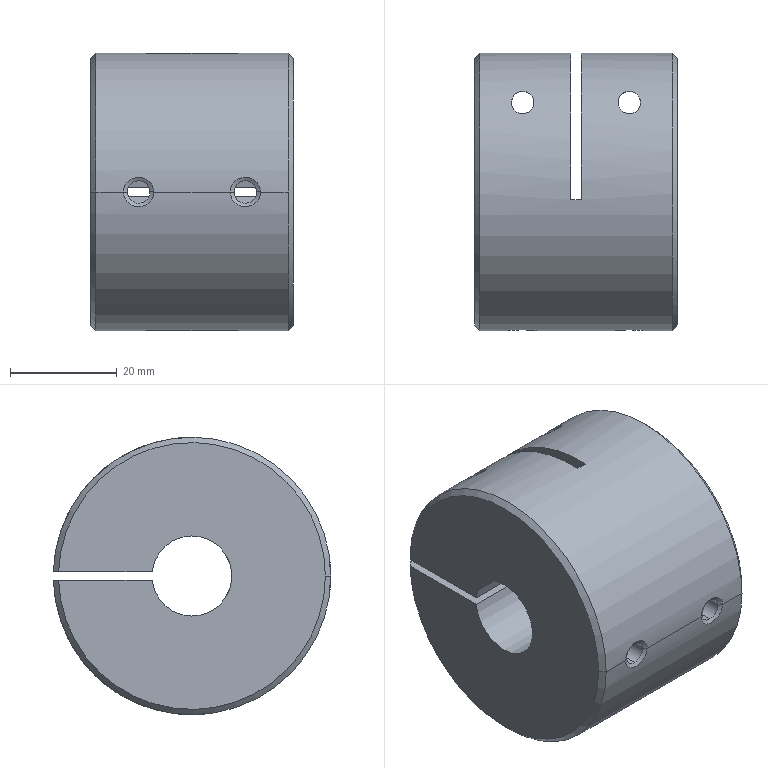Part | NX | 1 solid | 44 faces | box 38 x 51.989 x 52 mm | volume 66811 mm3 | cylinder 20 | plane 13 | cone 7 | spline 4 | commonest cylinder face diameters 4.2 x8 6 x4 10 x4 52 x2 15 x1 16 x1